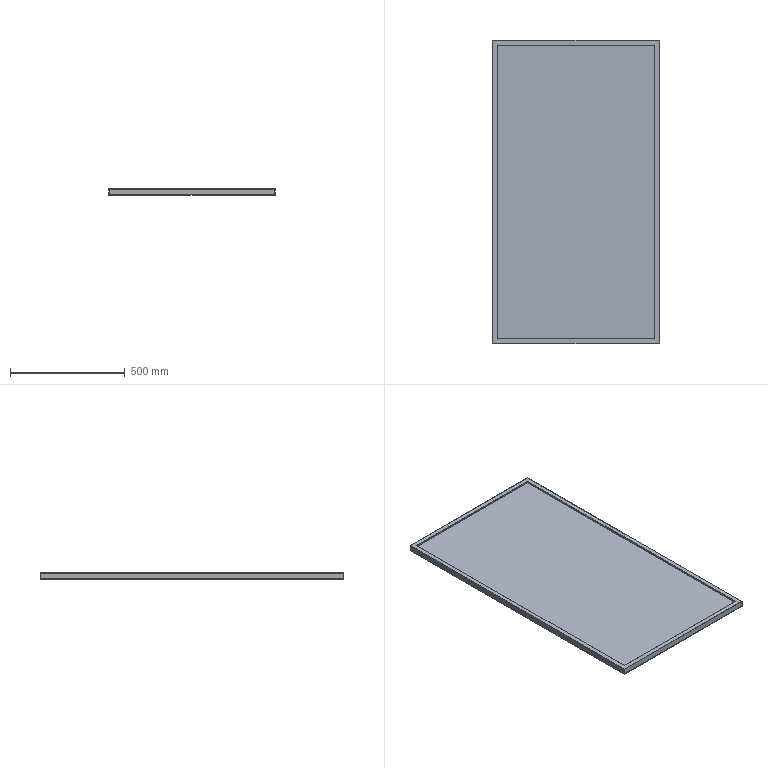Part | SolidWorks | features Extrusion 1, ICE 1, Shell 1 | 1 solid | 16 faces | box 724.5 x 1319 x 28 mm | volume 2267303 mm3 | plane 16
STEP:
#1=CARTESIAN_POINT('',(0.,1319.,28.));
#2=VERTEX_POINT('',#1);
#3=CARTESIAN_POINT('',(0.,0.,28.));
#4=VERTEX_POINT('',#3);
#5=CARTESIAN_POINT('',(0.,0.,28.));
#6=DIRECTION('',(0.,-1.,0.));
#7=VECTOR('',#6,1000.);
#8=LINE('',#5,#7);
#9=EDGE_CURVE('',#2,#4,#8,.T.);
#10=ORIENTED_EDGE('',*,*,#9,.T.);
#11=CARTESIAN_POINT('',(724.5,0.,28.));
#12=VERTEX_POINT('',#11);
#13=CARTESIAN_POINT('',(0.,0.,28.));
#14=DIRECTION('',(1.,0.,0.));
#15=VECTOR('',#14,1000.);
#16=LINE('',#13,#15);
#17=EDGE_CURVE('',#4,#12,#16,.T.);
#18=ORIENTED_EDGE('',*,*,#17,.T.);
#19=CARTESIAN_POINT('',(724.5,1319.,28.));
#20=VERTEX_POINT('',#19);
#21=CARTESIAN_POINT('',(724.5,0.,28.));
#22=DIRECTION('',(0.,1.,0.));
#23=VECTOR('',#22,1000.);
#24=LINE('',#21,#23);
#25=EDGE_CURVE('',#12,#20,#24,.T.);
#26=ORIENTED_EDGE('',*,*,#25,.T.);
#27=CARTESIAN_POINT('',(0.,1319.,28.));
#28=DIRECTION('',(-1.,0.,0.));
#29=VECTOR('',#28,1000.);
#30=LINE('',#27,#29);
#31=EDGE_CURVE('',#20,#2,#30,.T.);
#32=ORIENTED_EDGE('',*,*,#31,.T.);
#33=EDGE_LOOP('',(#10,#18,#26,#32));
#34=FACE_OUTER_BOUND('',#33,.T.);
#35=CARTESIAN_POINT('',(704.5,1299.,28.));
#36=VERTEX_POINT('',#35);
#37=CARTESIAN_POINT('',(20.,1299.,28.));
#38=VERTEX_POINT('',#37);
#39=CARTESIAN_POINT('',(704.5,1299.,28.));
#40=DIRECTION('',(-1.,0.,0.));
#41=VECTOR('',#40,1000.);
#42=LINE('',#39,#41);
#43=EDGE_CURVE('',#36,#38,#42,.T.);
#44=ORIENTED_EDGE('',*,*,#43,.F.);
#45=CARTESIAN_POINT('',(704.5,20.,28.));
#46=VERTEX_POINT('',#45);
#47=CARTESIAN_POINT('',(704.5,20.,28.));
#48=DIRECTION('',(0.,1.,0.));
#49=VECTOR('',#48,1000.);
#50=LINE('',#47,#49);
#51=EDGE_CURVE('',#46,#36,#50,.T.);
#52=ORIENTED_EDGE('',*,*,#51,.F.);
#53=CARTESIAN_POINT('',(20.,20.,28.));
#54=VERTEX_POINT('',#53);
#55=CARTESIAN_POINT('',(20.,20.,28.));
#56=DIRECTION('',(1.,0.,0.));
#57=VECTOR('',#56,1000.);
#58=LINE('',#55,#57);
#59=EDGE_CURVE('',#54,#46,#58,.T.);
#60=ORIENTED_EDGE('',*,*,#59,.F.);
#61=CARTESIAN_POINT('',(20.,1299.,28.));
#62=DIRECTION('',(0.,-1.,0.));
#63=VECTOR('',#62,1000.);
#64=LINE('',#61,#63);
#65=EDGE_CURVE('',#38,#54,#64,.T.);
#66=ORIENTED_EDGE('',*,*,#65,.F.);
#67=EDGE_LOOP('',(#44,#52,#60,#66));
#68=FACE_BOUND('',#67,.T.);
#69=CARTESIAN_POINT('',(0.,1319.,28.));
#70=DIRECTION('',(0.,0.,-1.));
#71=DIRECTION('',(-1.,0.,0.));
#72=AXIS2_PLACEMENT_3D('',#69,#70,#71);
#73=PLANE('',#72);
#74=ADVANCED_FACE('',(#34,#68),#73,.F.);
#75=CARTESIAN_POINT('',(0.,1319.,0.));
#76=VERTEX_POINT('',#75);
#77=CARTESIAN_POINT('',(0.,1319.,28.));
#78=DIRECTION('',(0.,0.,-1.));
#79=VECTOR('',#78,1000.);
#80=LINE('',#77,#79);
#81=EDGE_CURVE('',#2,#76,#80,.T.);
#82=ORIENTED_EDGE('',*,*,#81,.T.);
#83=CARTESIAN_POINT('',(0.,0.,0.));
#84=VERTEX_POINT('',#83);
#85=CARTESIAN_POINT('',(0.,0.,0.));
#86=DIRECTION('',(0.,-1.,0.));
#87=VECTOR('',#86,1000.);
#88=LINE('',#85,#87);
#89=EDGE_CURVE('',#76,#84,#88,.T.);
#90=ORIENTED_EDGE('',*,*,#89,.T.);
#91=CARTESIAN_POINT('',(0.,0.,28.));
#92=DIRECTION('',(0.,0.,-1.));
#93=VECTOR('',#92,1000.);
#94=LINE('',#91,#93);
#95=EDGE_CURVE('',#4,#84,#94,.T.);
#96=ORIENTED_EDGE('',*,*,#95,.F.);
#97=ORIENTED_EDGE('',*,*,#9,.F.);
#98=EDGE_LOOP('',(#82,#90,#96,#97));
#99=FACE_OUTER_BOUND('',#98,.T.);
#100=CARTESIAN_POINT('',(0.,0.,28.));
#101=DIRECTION('',(1.,0.,0.));
#102=DIRECTION('',(0.,0.,-1.));
#103=AXIS2_PLACEMENT_3D('',#100,#101,#102);
#104=PLANE('',#103);
#105=ADVANCED_FACE('',(#99),#104,.F.);
#106=ORIENTED_EDGE('',*,*,#95,.T.);
#107=CARTESIAN_POINT('',(724.5,0.,0.));
#108=VERTEX_POINT('',#107);
#109=CARTESIAN_POINT('',(0.,0.,0.));
#110=DIRECTION('',(1.,0.,0.));
#111=VECTOR('',#110,1000.);
#112=LINE('',#109,#111);
#113=EDGE_CURVE('',#84,#108,#112,.T.);
#114=ORIENTED_EDGE('',*,*,#113,.T.);
#115=CARTESIAN_POINT('',(724.5,0.,28.));
#116=DIRECTION('',(0.,0.,-1.));
#117=VECTOR('',#116,1000.);
#118=LINE('',#115,#117);
#119=EDGE_CURVE('',#12,#108,#118,.T.);
#120=ORIENTED_EDGE('',*,*,#119,.F.);
#121=ORIENTED_EDGE('',*,*,#17,.F.);
#122=EDGE_LOOP('',(#106,#114,#120,#121));
#123=FACE_OUTER_BOUND('',#122,.T.);
#124=CARTESIAN_POINT('',(0.,0.,28.));
#125=DIRECTION('',(0.,1.,0.));
#126=DIRECTION('',(0.,0.,1.));
#127=AXIS2_PLACEMENT_3D('',#124,#125,#126);
#128=PLANE('',#127);
#129=ADVANCED_FACE('',(#123),#128,.F.);
#130=ORIENTED_EDGE('',*,*,#119,.T.);
#131=CARTESIAN_POINT('',(724.5,1319.,0.));
#132=VERTEX_POINT('',#131);
#133=CARTESIAN_POINT('',(724.5,0.,0.));
#134=DIRECTION('',(0.,1.,0.));
#135=VECTOR('',#134,1000.);
#136=LINE('',#133,#135);
#137=EDGE_CURVE('',#108,#132,#136,.T.);
#138=ORIENTED_EDGE('',*,*,#137,.T.);
#139=CARTESIAN_POINT('',(724.5,1319.,28.));
#140=DIRECTION('',(0.,0.,-1.));
#141=VECTOR('',#140,1000.);
#142=LINE('',#139,#141);
#143=EDGE_CURVE('',#20,#132,#142,.T.);
#144=ORIENTED_EDGE('',*,*,#143,.F.);
#145=ORIENTED_EDGE('',*,*,#25,.F.);
#146=EDGE_LOOP('',(#130,#138,#144,#145));
#147=FACE_OUTER_BOUND('',#146,.T.);
#148=CARTESIAN_POINT('',(724.5,0.,28.));
#149=DIRECTION('',(-1.,0.,0.));
#150=DIRECTION('',(0.,0.,1.));
#151=AXIS2_PLACEMENT_3D('',#148,#149,#150);
#152=PLANE('',#151);
#153=ADVANCED_FACE('',(#147),#152,.F.);
#154=ORIENTED_EDGE('',*,*,#143,.T.);
#155=CARTESIAN_POINT('',(0.,1319.,0.));
#156=DIRECTION('',(-1.,0.,0.));
#157=VECTOR('',#156,1000.);
#158=LINE('',#155,#157);
#159=EDGE_CURVE('',#132,#76,#158,.T.);
#160=ORIENTED_EDGE('',*,*,#159,.T.);
#161=ORIENTED_EDGE('',*,*,#81,.F.);
#162=ORIENTED_EDGE('',*,*,#31,.F.);
#163=EDGE_LOOP('',(#154,#160,#161,#162));
#164=FACE_OUTER_BOUND('',#163,.T.);
#165=CARTESIAN_POINT('',(0.,1319.,28.));
#166=DIRECTION('',(0.,-1.,0.));
#167=DIRECTION('',(0.,0.,-1.));
#168=AXIS2_PLACEMENT_3D('',#165,#166,#167);
#169=PLANE('',#168);
#170=ADVANCED_FACE('',(#164),#169,.F.);
#171=ORIENTED_EDGE('',*,*,#89,.F.);
#172=ORIENTED_EDGE('',*,*,#159,.F.);
#173=ORIENTED_EDGE('',*,*,#137,.F.);
#174=ORIENTED_EDGE('',*,*,#113,.F.);
#175=EDGE_LOOP('',(#171,#172,#173,#174));
#176=FACE_OUTER_BOUND('',#175,.T.);
#177=CARTESIAN_POINT('',(0.,1319.,0.));
#178=DIRECTION('',(0.,0.,-1.));
#179=DIRECTION('',(-1.,0.,0.));
#180=AXIS2_PLACEMENT_3D('',#177,#178,#179);
#181=PLANE('',#180);
#182=ADVANCED_FACE('',(#176),#181,.T.);
#183=CARTESIAN_POINT('',(2.,1317.,26.));
#184=VERTEX_POINT('',#183);
#185=CARTESIAN_POINT('',(2.,2.,26.));
#186=VERTEX_POINT('',#185);
#187=CARTESIAN_POINT('',(2.,0.,26.));
#188=DIRECTION('',(0.,-1.,0.));
#189=VECTOR('',#188,1000.);
#190=LINE('',#187,#189);
#191=EDGE_CURVE('',#184,#186,#190,.T.);
#192=ORIENTED_EDGE('',*,*,#191,.F.);
#193=CARTESIAN_POINT('',(722.5,1317.,26.));
#194=VERTEX_POINT('',#193);
#195=CARTESIAN_POINT('',(0.,1317.,26.));
#196=DIRECTION('',(-1.,0.,0.));
#197=VECTOR('',#196,1000.);
#198=LINE('',#195,#197);
#199=EDGE_CURVE('',#194,#184,#198,.T.);
#200=ORIENTED_EDGE('',*,*,#199,.F.);
#201=CARTESIAN_POINT('',(722.5,2.,26.));
#202=VERTEX_POINT('',#201);
#203=CARTESIAN_POINT('',(722.5,0.,26.));
#204=DIRECTION('',(0.,1.,0.));
#205=VECTOR('',#204,1000.);
#206=LINE('',#203,#205);
#207=EDGE_CURVE('',#202,#194,#206,.T.);
#208=ORIENTED_EDGE('',*,*,#207,.F.);
#209=CARTESIAN_POINT('',(0.,2.,26.));
#210=DIRECTION('',(1.,0.,0.));
#211=VECTOR('',#210,1000.);
#212=LINE('',#209,#211);
#213=EDGE_CURVE('',#186,#202,#212,.T.);
#214=ORIENTED_EDGE('',*,*,#213,.F.);
#215=EDGE_LOOP('',(#192,#200,#208,#214));
#216=FACE_OUTER_BOUND('',#215,.T.);
#217=CARTESIAN_POINT('',(704.5,20.,26.));
#218=VERTEX_POINT('',#217);
#219=CARTESIAN_POINT('',(704.5,1299.,26.));
#220=VERTEX_POINT('',#219);
#221=CARTESIAN_POINT('',(704.5,20.,26.));
#222=DIRECTION('',(0.,1.,0.));
#223=VECTOR('',#222,1000.);
#224=LINE('',#221,#223);
#225=EDGE_CURVE('',#218,#220,#224,.T.);
#226=ORIENTED_EDGE('',*,*,#225,.T.);
#227=CARTESIAN_POINT('',(20.,1299.,26.));
#228=VERTEX_POINT('',#227);
#229=CARTESIAN_POINT('',(704.5,1299.,26.));
#230=DIRECTION('',(-1.,0.,0.));
#231=VECTOR('',#230,1000.);
#232=LINE('',#229,#231);
#233=EDGE_CURVE('',#220,#228,#232,.T.);
#234=ORIENTED_EDGE('',*,*,#233,.T.);
#235=CARTESIAN_POINT('',(20.,20.,26.));
#236=VERTEX_POINT('',#235);
#237=CARTESIAN_POINT('',(20.,1299.,26.));
#238=DIRECTION('',(0.,-1.,0.));
#239=VECTOR('',#238,1000.);
#240=LINE('',#237,#239);
#241=EDGE_CURVE('',#228,#236,#240,.T.);
#242=ORIENTED_EDGE('',*,*,#241,.T.);
#243=CARTESIAN_POINT('',(20.,20.,26.));
#244=DIRECTION('',(1.,0.,0.));
#245=VECTOR('',#244,1000.);
#246=LINE('',#243,#245);
#247=EDGE_CURVE('',#236,#218,#246,.T.);
#248=ORIENTED_EDGE('',*,*,#247,.T.);
#249=EDGE_LOOP('',(#226,#234,#242,#248));
#250=FACE_BOUND('',#249,.T.);
#251=CARTESIAN_POINT('',(0.,1319.,26.));
#252=DIRECTION('',(0.,0.,1.));
#253=DIRECTION('',(1.,0.,0.));
#254=AXIS2_PLACEMENT_3D('',#251,#252,#253);
#255=PLANE('',#254);
#256=ADVANCED_FACE('',(#216,#250),#255,.F.);
#257=ORIENTED_EDGE('',*,*,#43,.T.);
#258=CARTESIAN_POINT('',(20.,1299.,26.));
#259=DIRECTION('',(0.,0.,1.));
#260=VECTOR('',#259,1000.);
#261=LINE('',#258,#260);
#262=EDGE_CURVE('',#228,#38,#261,.T.);
#263=ORIENTED_EDGE('',*,*,#262,.F.);
#264=ORIENTED_EDGE('',*,*,#233,.F.);
#265=CARTESIAN_POINT('',(704.5,1299.,26.));
#266=DIRECTION('',(0.,0.,1.));
#267=VECTOR('',#266,1000.);
#268=LINE('',#265,#267);
#269=EDGE_CURVE('',#220,#36,#268,.T.);
#270=ORIENTED_EDGE('',*,*,#269,.T.);
#271=EDGE_LOOP('',(#257,#263,#264,#270));
#272=FACE_OUTER_BOUND('',#271,.T.);
#273=CARTESIAN_POINT('',(704.5,1299.,26.));
#274=DIRECTION('',(0.,1.,0.));
#275=DIRECTION('',(0.,0.,1.));
#276=AXIS2_PLACEMENT_3D('',#273,#274,#275);
#277=PLANE('',#276);
#278=ADVANCED_FACE('',(#272),#277,.F.);
#279=ORIENTED_EDGE('',*,*,#51,.T.);
#280=ORIENTED_EDGE('',*,*,#269,.F.);
#281=ORIENTED_EDGE('',*,*,#225,.F.);
#282=CARTESIAN_POINT('',(704.5,20.,26.));
#283=DIRECTION('',(0.,0.,1.));
#284=VECTOR('',#283,1000.);
#285=LINE('',#282,#284);
#286=EDGE_CURVE('',#218,#46,#285,.T.);
#287=ORIENTED_EDGE('',*,*,#286,.T.);
#288=EDGE_LOOP('',(#279,#280,#281,#287));
#289=FACE_OUTER_BOUND('',#288,.T.);
#290=CARTESIAN_POINT('',(704.5,20.,26.));
#291=DIRECTION('',(1.,0.,0.));
#292=DIRECTION('',(0.,0.,-1.));
#293=AXIS2_PLACEMENT_3D('',#290,#291,#292);
#294=PLANE('',#293);
#295=ADVANCED_FACE('',(#289),#294,.F.);
#296=ORIENTED_EDGE('',*,*,#59,.T.);
#297=ORIENTED_EDGE('',*,*,#286,.F.);
#298=ORIENTED_EDGE('',*,*,#247,.F.);
#299=CARTESIAN_POINT('',(20.,20.,26.));
#300=DIRECTION('',(0.,0.,1.));
#301=VECTOR('',#300,1000.);
#302=LINE('',#299,#301);
#303=EDGE_CURVE('',#236,#54,#302,.T.);
#304=ORIENTED_EDGE('',*,*,#303,.T.);
#305=EDGE_LOOP('',(#296,#297,#298,#304));
#306=FACE_OUTER_BOUND('',#305,.T.);
#307=CARTESIAN_POINT('',(20.,20.,26.));
#308=DIRECTION('',(0.,-1.,0.));
#309=DIRECTION('',(0.,0.,-1.));
#310=AXIS2_PLACEMENT_3D('',#307,#308,#309);
#311=PLANE('',#310);
#312=ADVANCED_FACE('',(#306),#311,.F.);
#313=ORIENTED_EDGE('',*,*,#65,.T.);
#314=ORIENTED_EDGE('',*,*,#303,.F.);
#315=ORIENTED_EDGE('',*,*,#241,.F.);
#316=ORIENTED_EDGE('',*,*,#262,.T.);
#317=EDGE_LOOP('',(#313,#314,#315,#316));
#318=FACE_OUTER_BOUND('',#317,.T.);
#319=CARTESIAN_POINT('',(20.,1299.,26.));
#320=DIRECTION('',(-1.,0.,0.));
#321=DIRECTION('',(0.,0.,1.));
#322=AXIS2_PLACEMENT_3D('',#319,#320,#321);
#323=PLANE('',#322);
#324=ADVANCED_FACE('',(#318),#323,.F.);
#325=CARTESIAN_POINT('',(2.,1317.,2.));
#326=VERTEX_POINT('',#325);
#327=CARTESIAN_POINT('',(2.,2.,2.));
#328=VERTEX_POINT('',#327);
#329=CARTESIAN_POINT('',(2.,1319.,2.));
#330=DIRECTION('',(0.,-1.,0.));
#331=VECTOR('',#330,1000.);
#332=LINE('',#329,#331);
#333=EDGE_CURVE('',#326,#328,#332,.T.);
#334=ORIENTED_EDGE('',*,*,#333,.T.);
#335=CARTESIAN_POINT('',(722.5,2.,2.));
#336=VERTEX_POINT('',#335);
#337=CARTESIAN_POINT('',(0.,2.,2.));
#338=DIRECTION('',(1.,0.,0.));
#339=VECTOR('',#338,1000.);
#340=LINE('',#337,#339);
#341=EDGE_CURVE('',#328,#336,#340,.T.);
#342=ORIENTED_EDGE('',*,*,#341,.T.);
#343=CARTESIAN_POINT('',(722.5,1317.,2.));
#344=VERTEX_POINT('',#343);
#345=CARTESIAN_POINT('',(722.5,1319.,2.));
#346=DIRECTION('',(0.,1.,0.));
#347=VECTOR('',#346,1000.);
#348=LINE('',#345,#347);
#349=EDGE_CURVE('',#336,#344,#348,.T.);
#350=ORIENTED_EDGE('',*,*,#349,.T.);
#351=CARTESIAN_POINT('',(0.,1317.,2.));
#352=DIRECTION('',(-1.,0.,0.));
#353=VECTOR('',#352,1000.);
#354=LINE('',#351,#353);
#355=EDGE_CURVE('',#344,#326,#354,.T.);
#356=ORIENTED_EDGE('',*,*,#355,.T.);
#357=EDGE_LOOP('',(#334,#342,#350,#356));
#358=FACE_OUTER_BOUND('',#357,.T.);
#359=CARTESIAN_POINT('',(0.,1319.,2.));
#360=DIRECTION('',(0.,0.,-1.));
#361=DIRECTION('',(-1.,0.,0.));
#362=AXIS2_PLACEMENT_3D('',#359,#360,#361);
#363=PLANE('',#362);
#364=ADVANCED_FACE('',(#358),#363,.F.);
#365=CARTESIAN_POINT('',(722.5,1317.,28.));
#366=DIRECTION('',(0.,0.,-1.));
#367=VECTOR('',#366,1000.);
#368=LINE('',#365,#367);
#369=EDGE_CURVE('',#194,#344,#368,.T.);
#370=ORIENTED_EDGE('',*,*,#369,.F.);
#371=ORIENTED_EDGE('',*,*,#199,.T.);
#372=CARTESIAN_POINT('',(2.,1317.,28.));
#373=DIRECTION('',(0.,0.,-1.));
#374=VECTOR('',#373,1000.);
#375=LINE('',#372,#374);
#376=EDGE_CURVE('',#184,#326,#375,.T.);
#377=ORIENTED_EDGE('',*,*,#376,.T.);
#378=ORIENTED_EDGE('',*,*,#355,.F.);
#379=EDGE_LOOP('',(#370,#371,#377,#378));
#380=FACE_OUTER_BOUND('',#379,.T.);
#381=CARTESIAN_POINT('',(0.,1317.,28.));
#382=DIRECTION('',(0.,-1.,0.));
#383=DIRECTION('',(0.,0.,-1.));
#384=AXIS2_PLACEMENT_3D('',#381,#382,#383);
#385=PLANE('',#384);
#386=ADVANCED_FACE('',(#380),#385,.T.);
#387=CARTESIAN_POINT('',(722.5,2.,28.));
#388=DIRECTION('',(0.,0.,-1.));
#389=VECTOR('',#388,1000.);
#390=LINE('',#387,#389);
#391=EDGE_CURVE('',#202,#336,#390,.T.);
#392=ORIENTED_EDGE('',*,*,#391,.F.);
#393=ORIENTED_EDGE('',*,*,#207,.T.);
#394=ORIENTED_EDGE('',*,*,#369,.T.);
#395=ORIENTED_EDGE('',*,*,#349,.F.);
#396=EDGE_LOOP('',(#392,#393,#394,#395));
#397=FACE_OUTER_BOUND('',#396,.T.);
#398=CARTESIAN_POINT('',(722.5,0.,28.));
#399=DIRECTION('',(-1.,0.,0.));
#400=DIRECTION('',(0.,0.,1.));
#401=AXIS2_PLACEMENT_3D('',#398,#399,#400);
#402=PLANE('',#401);
#403=ADVANCED_FACE('',(#397),#402,.T.);
#404=CARTESIAN_POINT('',(2.,2.,28.));
#405=DIRECTION('',(0.,0.,-1.));
#406=VECTOR('',#405,1000.);
#407=LINE('',#404,#406);
#408=EDGE_CURVE('',#186,#328,#407,.T.);
#409=ORIENTED_EDGE('',*,*,#408,.F.);
#410=ORIENTED_EDGE('',*,*,#213,.T.);
#411=ORIENTED_EDGE('',*,*,#391,.T.);
#412=ORIENTED_EDGE('',*,*,#341,.F.);
#413=EDGE_LOOP('',(#409,#410,#411,#412));
#414=FACE_OUTER_BOUND('',#413,.T.);
#415=CARTESIAN_POINT('',(0.,2.,28.));
#416=DIRECTION('',(0.,1.,0.));
#417=DIRECTION('',(0.,0.,1.));
#418=AXIS2_PLACEMENT_3D('',#415,#416,#417);
#419=PLANE('',#418);
#420=ADVANCED_FACE('',(#414),#419,.T.);
#421=ORIENTED_EDGE('',*,*,#376,.F.);
#422=ORIENTED_EDGE('',*,*,#191,.T.);
#423=ORIENTED_EDGE('',*,*,#408,.T.);
#424=ORIENTED_EDGE('',*,*,#333,.F.);
#425=EDGE_LOOP('',(#421,#422,#423,#424));
#426=FACE_OUTER_BOUND('',#425,.T.);
#427=CARTESIAN_POINT('',(2.,0.,28.));
#428=DIRECTION('',(1.,0.,0.));
#429=DIRECTION('',(0.,0.,-1.));
#430=AXIS2_PLACEMENT_3D('',#427,#428,#429);
#431=PLANE('',#430);
#432=ADVANCED_FACE('',(#426),#431,.T.);
#433=CLOSED_SHELL('',(#74,#105,#129,#153,#170,#182,#256,#278,#295,#312,#324,#364,#386,#403,#420,#432));
#434=MANIFOLD_SOLID_BREP('',#433);
#435=CARTESIAN_POINT('',(0.,0.,0.));
#436=DIRECTION('',(0.,0.,1.));
#437=DIRECTION('',(1.,0.,0.));
#438=AXIS2_PLACEMENT_3D('',#435,#436,#437);
#439=(LENGTH_UNIT()NAMED_UNIT(*)SI_UNIT(.MILLI.,.METRE.));
#440=UNCERTAINTY_MEASURE_WITH_UNIT(LENGTH_MEASURE(0.00001),#439,'','');
#441=(NAMED_UNIT(*)PLANE_ANGLE_UNIT()SI_UNIT($,.RADIAN.));
#442=(NAMED_UNIT(*)SI_UNIT($,.STERADIAN.)SOLID_ANGLE_UNIT());
#443=(GEOMETRIC_REPRESENTATION_CONTEXT(3)GLOBAL_UNCERTAINTY_ASSIGNED_CONTEXT((#440))GLOBAL_UNIT_ASSIGNED_CONTEXT((#439,#441,#442))REPRESENTATION_CONTEXT('',''));
#444=ADVANCED_BREP_SHAPE_REPRESENTATION('',(#434,#438),#443);